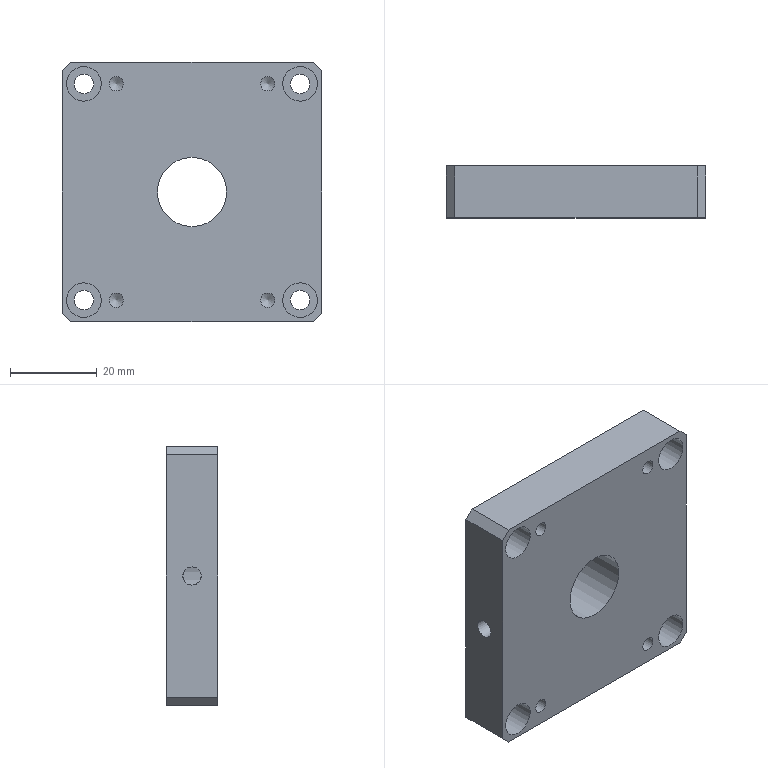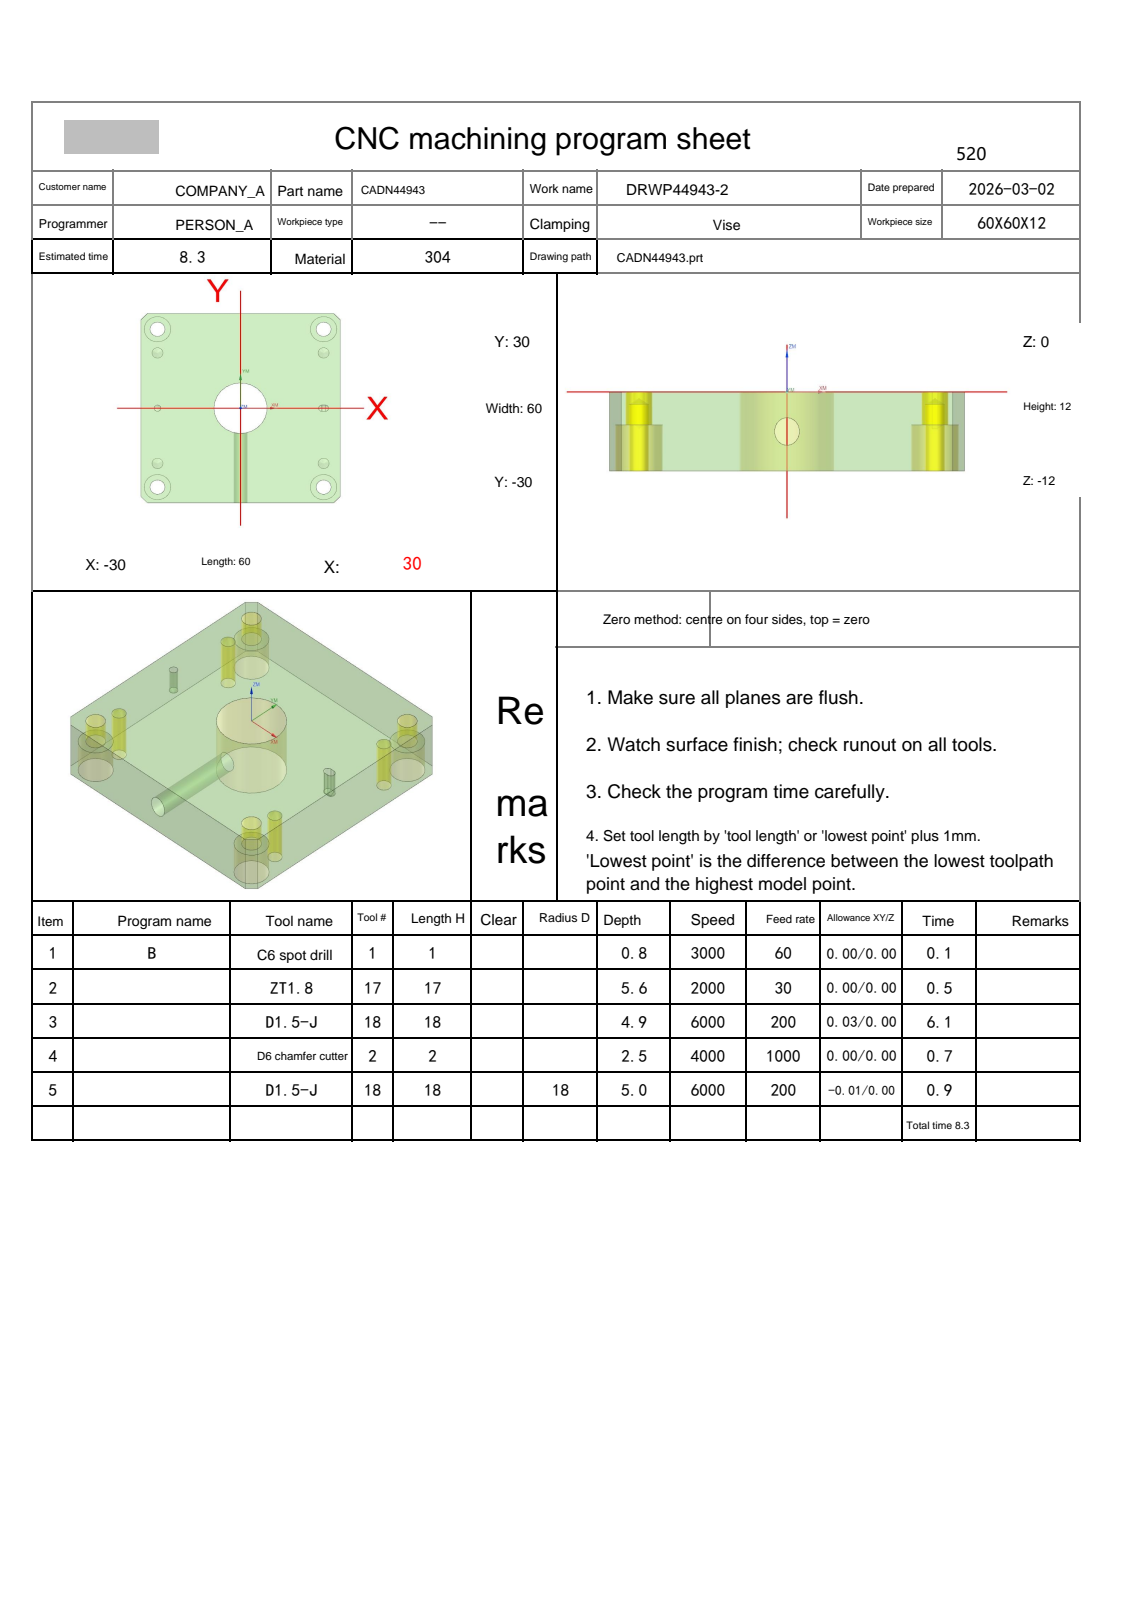NC program | NX | posted by the shop | part box 60 x 12 x 60 mm
Lines 2670 to 3254 of 3254:
N4 T02 M06
(D6 chamfer cutter  D=6. R=0. H=02 ce=0.00 di=0.00)
G00 G90 G54 X-25. Y-25. M03 S2000
G43 H02 Z50.
M08
G98 G81 X-25. Y-25. Z-2.55 R3. F100.
Y25.
X25.
Y-25.
G80
G00 Z50.
G00 G90 X-.386 Y31.227 M03 S3500
Z50.
Z.172
G01 Z-1.2 F1000.
G03 X-.1 Y31.027 I1.286 J1.532
G01 X-.054 Y30.997
X0.0 Y31.
X28.
X28.259 Y30.966
X28.5 Y30.866
X28.707 Y30.707
X30.707 Y28.707
X30.866 Y28.5
X30.966 Y28.259
X31. Y28.
Y-28.
X30.966 Y-28.259
X30.866 Y-28.5
X30.707 Y-28.707
X28.707 Y-30.707
X28.5 Y-30.866
X28.259 Y-30.966
X28. Y-31.
X-28.
X-28.259 Y-30.966
X-28.5 Y-30.866
X-28.707 Y-30.707
X-30.707 Y-28.707
X-30.866 Y-28.5
X-30.966 Y-28.259
X-31. Y-28.
Y28.
X-30.966 Y28.259
X-30.866 Y28.5
X-30.707 Y28.707
X-28.707 Y30.707
X-28.5 Y30.866
X-28.259 Y30.966
X-28. Y31.
X0.0
X.054 Y30.997
X.1 Y31.027
G03 X.386 Y31.227 I-1. J1.732
G01 Z.172
G00 Z10.
X-26.065 Y25.407
Z.294
G01 Z-1.2
G03 X-26.234 Y25.102 I1.658 J-1.118
G01 X-26.259 Y25.054
X-26.25 Y25.
G03 X-25. Y23.75 I1.25 J0.0
X-23.75 Y25. I0.0 J1.25
X-25. Y26.25 I-1.25 J0.0
X-26.223 Y25.26 I0.0 J-1.25
G01 X-26.25 Y25.
X-26.259 Y24.946
X-26.234 Y24.898
G03 X-26.065 Y24.593 I1.827 J.813
G01 Z.294
G00 Z10.
X23.935 Y25.407
Z.294
G01 Z-1.2
G03 X23.766 Y25.102 I1.658 J-1.118
G01 X23.741 Y25.054
X23.75 Y25.
G03 X25. Y23.75 I1.25 J0.0
X26.25 Y25. I0.0 J1.25
X25. Y26.25 I-1.25 J0.0
X23.777 Y25.26 I0.0 J-1.25
G01 X23.75 Y25.
X23.741 Y24.946
X23.766 Y24.898
G03 X23.935 Y24.593 I1.827 J.813
G01 Z.294
G00 Z10.
X25.116 Y-.068
Z.467
G01 Z-1.2
X25.03 Y-.008
X25. Y0.0
X24.5
X25.5
X25.
X24.97 Y-.008
X24.884 Y-.068
Z.467
G00 Z10.
X23.935 Y-24.593
Z.294
G01 Z-1.2
G03 X23.766 Y-24.898 I1.658 J-1.118
G01 X23.741 Y-24.946
X23.75 Y-25.
G03 X25. Y-26.25 I1.25 J0.0
X26.25 Y-25. I0.0 J1.25
X25. Y-23.75 I-1.25 J0.0
X23.777 Y-24.74 I0.0 J-1.25
G01 X23.75 Y-25.
X23.741 Y-25.054
X23.766 Y-25.102
G03 X23.935 Y-25.407 I1.827 J.813
G01 Z.294
G00 Z10.
X6.794 Y-.397
Z.208
G01 Z-1.2
G03 X6.978 Y-.101 I-1.597 J1.204
G01 X7.006 Y-.054
X7. Y0.0
G03 X0.0 Y7. I-7. J0.0
X-7. Y0.0 I0.0 J-7.
X0.0 Y-7. I7. J0.0
X7. Y0.0 I0.0 J7.
G01 X7.006 Y.054
X6.978 Y.101
G03 X6.794 Y.397 I-1.782 J-.908
G01 Z.208
G00 Z10.
X-26.065 Y-24.593
Z.294
G01 Z-1.2
G03 X-26.234 Y-24.898 I1.658 J-1.118
G01 X-26.259 Y-24.946
X-26.25 Y-25.
G03 X-25. Y-26.25 I1.25 J0.0
X-23.75 Y-25. I0.0 J1.25
X-25. Y-23.75 I-1.25 J0.0
X-26.223 Y-24.74 I0.0 J-1.25
G01 X-26.25 Y-25.
X-26.259 Y-25.054
X-26.234 Y-25.102
G03 X-26.065 Y-25.407 I1.827 J.813
G01 Z.294
G00 Z50.
G00 G90 X-25. Y0.0 M03 S4000
Z50.
G98 G81 X-25. Y0.0 Z-1.3 R3. F80.
G80
G00 Z50.
G91 G28 Z0.0
M05
M09
G91 G28 Z0.0
M01
N5 T18 M06
(D1.5-J  D=1.5 R=0. H=18 ce=-0.01 di=0.00)
G00 G90 G54 X25.254 Y-.227 M03 S6000
G43 H18 Z50.
M08
Z.5
G01 X25.548 Z.485 F200.
X25.664 Y-.164 Z.478
X25.727 Y-.048 Z.471
Y.048 Z.466
X25.664 Y.164 Z.459
X25.548 Y.227 Z.452
X24.452 Z.394
X24.336 Y.164 Z.387
X24.273 Y.048 Z.38
Y-.048 Z.375
X24.323 Y-.151 Z.369
X24.417 Y-.217 Z.363
X24.5 Y-.227 Z.359
X25.548 Z.304
X25.664 Y-.164 Z.297
X25.727 Y-.048 Z.29
Y.048 Z.285
X25.664 Y.164 Z.278
X25.548 Y.227 Z.271
X24.452 Z.214
X24.336 Y.164 Z.207
X24.273 Y.048 Z.2
Y-.048 Z.195
X24.323 Y-.151 Z.189
X24.417 Y-.217 Z.183
X24.5 Y-.227 Z.179
X25.548 Z.124
X25.664 Y-.164 Z.117
X25.727 Y-.048 Z.11
Y.048 Z.105
X25.664 Y.164 Z.098
X25.548 Y.227 Z.091
X24.452 Z.033
X24.336 Y.164 Z.027
X24.273 Y.048 Z.02
Y-.048 Z.015
X24.323 Y-.151 Z.009
X24.417 Y-.217 Z.003
X24.465 Y-.225 Z0.0
G41 D18
X24.5 Y-.26
X25.5 Z-.053
G03 X25.76 Y0.0 Z-.075 I0.0 J.26
X25.5 Y.26 Z-.096 I-.26 J0.0
G01 X24.5 Z-.149
G03 X24.24 Y0.0 Z-.171 I0.0 J-.26
X24.5 Y-.26 Z-.192 I.26 J0.0
G01 X25.5 Z-.245
G03 X25.76 Y0.0 Z-.267 I0.0 J.26
X25.5 Y.26 Z-.288 I-.26 J0.0
G01 X24.5 Z-.341
G03 X24.24 Y0.0 Z-.363 I0.0 J-.26
X24.5 Y-.26 Z-.385 I.26 J0.0
G01 X25.5 Z-.438
G03 X25.76 Y0.0 Z-.459 I0.0 J.26
X25.5 Y.26 Z-.481 I-.26 J0.0
G01 X24.5 Z-.534
G03 X24.24 Y0.0 Z-.555 I0.0 J-.26
X24.5 Y-.26 Z-.577 I.26 J0.0
G01 X25.5 Z-.63
G03 X25.76 Y0.0 Z-.651 I0.0 J.26
X25.5 Y.26 Z-.673 I-.26 J0.0
G01 X24.5 Z-.726
G03 X24.24 Y0.0 Z-.748 I0.0 J-.26
X24.5 Y-.26 Z-.769 I.26 J0.0
G01 X25.5 Z-.822
G03 X25.76 Y0.0 Z-.844 I0.0 J.26
X25.5 Y.26 Z-.865 I-.26 J0.0
G01 X24.5 Z-.918
G03 X24.24 Y0.0 Z-.94 I0.0 J-.26
X24.5 Y-.26 Z-.962 I.26 J0.0
G01 X25.5 Z-1.014
G03 X25.76 Y0.0 Z-1.036 I0.0 J.26
X25.5 Y.26 Z-1.058 I-.26 J0.0
G01 X24.5 Z-1.111
G03 X24.24 Y0.0 Z-1.132 I0.0 J-.26
X24.5 Y-.26 Z-1.154 I.26 J0.0
G01 X25.5 Z-1.207
G03 X25.76 Y0.0 Z-1.228 I0.0 J.26
X25.5 Y.26 Z-1.25 I-.26 J0.0
G01 X24.5 Z-1.303
G03 X24.24 Y0.0 Z-1.325 I0.0 J-.26
X24.5 Y-.26 Z-1.346 I.26 J0.0
G01 X25.5 Z-1.399
G03 X25.76 Y0.0 Z-1.421 I0.0 J.26
X25.5 Y.26 Z-1.442 I-.26 J0.0
G01 X24.5 Z-1.495
G03 X24.24 Y0.0 Z-1.517 I0.0 J-.26
X24.5 Y-.26 Z-1.538 I.26 J0.0
G01 X25.5 Z-1.591
G03 X25.76 Y0.0 Z-1.613 I0.0 J.26
X25.5 Y.26 Z-1.635 I-.26 J0.0
G01 X24.5 Z-1.688
G03 X24.24 Y0.0 Z-1.709 I0.0 J-.26
X24.5 Y-.26 Z-1.731 I.26 J0.0
G01 X25.5 Z-1.784
G03 X25.76 Y0.0 Z-1.805 I0.0 J.26
X25.5 Y.26 Z-1.827 I-.26 J0.0
G01 X24.5 Z-1.88
G03 X24.24 Y0.0 Z-1.901 I0.0 J-.26
X24.5 Y-.26 Z-1.923 I.26 J0.0
G01 X25.5 Z-1.976
G03 X25.76 Y0.0 Z-1.998 I0.0 J.26
X25.5 Y.26 Z-2.019 I-.26 J0.0
G01 X24.5 Z-2.072
G03 X24.24 Y0.0 Z-2.094 I0.0 J-.26
X24.5 Y-.26 Z-2.115 I.26 J0.0
G01 X25.5 Z-2.168
G03 X25.76 Y0.0 Z-2.19 I0.0 J.26
X25.5 Y.26 Z-2.212 I-.26 J0.0
G01 X24.5 Z-2.264
G03 X24.24 Y0.0 Z-2.286 I0.0 J-.26
X24.5 Y-.26 Z-2.308 I.26 J0.0
G01 X25.5 Z-2.361
G03 X25.76 Y0.0 Z-2.382 I0.0 J.26
X25.5 Y.26 Z-2.404 I-.26 J0.0
G01 X24.5 Z-2.457
G03 X24.24 Y0.0 Z-2.478 I0.0 J-.26
X24.5 Y-.26 Z-2.5 I.26 J0.0
G01 X25.5 Z-2.553
G03 X25.76 Y0.0 Z-2.575 I0.0 J.26
X25.5 Y.26 Z-2.596 I-.26 J0.0
G01 X24.5 Z-2.649
G03 X24.24 Y0.0 Z-2.671 I0.0 J-.26
X24.5 Y-.26 Z-2.692 I.26 J0.0
G01 X25.5 Z-2.745
G03 X25.76 Y0.0 Z-2.767 I0.0 J.26
X25.5 Y.26 Z-2.788 I-.26 J0.0
G01 X24.5 Z-2.841
G03 X24.24 Y0.0 Z-2.863 I0.0 J-.26
X24.5 Y-.26 Z-2.885 I.26 J0.0
G01 X25.5 Z-2.938
G03 X25.76 Y0.0 Z-2.959 I0.0 J.26
X25.5 Y.26 Z-2.981 I-.26 J0.0
G01 X24.5 Z-3.034
G03 X24.24 Y0.0 Z-3.055 I0.0 J-.26
X24.5 Y-.26 Z-3.077 I.26 J0.0
G01 X25.5 Z-3.13
G03 X25.76 Y0.0 Z-3.151 I0.0 J.26
X25.5 Y.26 Z-3.173 I-.26 J0.0
G01 X24.5 Z-3.226
G03 X24.24 Y0.0 Z-3.248 I0.0 J-.26
X24.5 Y-.26 Z-3.269 I.26 J0.0
G01 X25.5 Z-3.322
G03 X25.76 Y0.0 Z-3.344 I0.0 J.26
X25.5 Y.26 Z-3.365 I-.26 J0.0
G01 X24.5 Z-3.418
G03 X24.24 Y0.0 Z-3.44 I0.0 J-.26
X24.5 Y-.26 Z-3.462 I.26 J0.0
G01 X25.5 Z-3.514
G03 X25.76 Y0.0 Z-3.536 I0.0 J.26
X25.5 Y.26 Z-3.558 I-.26 J0.0
G01 X24.5 Z-3.611
G03 X24.24 Y0.0 Z-3.632 I0.0 J-.26
X24.5 Y-.26 Z-3.654 I.26 J0.0
G01 X25.5 Z-3.707
G03 X25.76 Y0.0 Z-3.728 I0.0 J.26
X25.5 Y.26 Z-3.75 I-.26 J0.0
G01 X24.5 Z-3.803
G03 X24.24 Y0.0 Z-3.825 I0.0 J-.26
X24.5 Y-.26 Z-3.846 I.26 J0.0
G01 X25.5 Z-3.899
G03 X25.76 Y0.0 Z-3.921 I0.0 J.26
X25.5 Y.26 Z-3.942 I-.26 J0.0
G01 X24.5 Z-3.995
G03 X24.24 Y0.0 Z-4.017 I0.0 J-.26
X24.5 Y-.26 Z-4.038 I.26 J0.0
G01 X25.5 Z-4.091
G03 X25.76 Y0.0 Z-4.113 I0.0 J.26
X25.5 Y.26 Z-4.135 I-.26 J0.0
G01 X24.5 Z-4.188
G03 X24.24 Y0.0 Z-4.209 I0.0 J-.26
X24.5 Y-.26 Z-4.231 I.26 J0.0
G01 X25.5 Z-4.284
G03 X25.76 Y0.0 Z-4.305 I0.0 J.26
X25.5 Y.26 Z-4.327 I-.26 J0.0
G01 X24.5 Z-4.38
G03 X24.24 Y0.0 Z-4.401 I0.0 J-.26
X24.5 Y-.26 Z-4.423 I.26 J0.0
G01 X25.5 Z-4.476
G03 X25.76 Y0.0 Z-4.498 I0.0 J.26
X25.5 Y.26 Z-4.519 I-.26 J0.0
G01 X24.5 Z-4.572
G03 X24.24 Y0.0 Z-4.594 I0.0 J-.26
X24.5 Y-.26 Z-4.615 I.26 J0.0
G01 X25.5 Z-4.668
G03 X25.76 Y0.0 Z-4.69 I0.0 J.26
X25.5 Y.26 Z-4.712 I-.26 J0.0
G01 X24.5 Z-4.764
G03 X24.24 Y0.0 Z-4.786 I0.0 J-.26
X24.5 Y-.26 Z-4.808 I.26 J0.0
G01 X25.5 Z-4.861
G03 X25.76 Y0.0 Z-4.882 I0.0 J.26
X25.5 Y.26 Z-4.904 I-.26 J0.0
G01 X24.5 Z-4.957
G03 X24.24 Y0.0 Z-4.978 I0.0 J-.26
X24.5 Y-.26 Z-5. I.26 J0.0
G01 X25.5
G03 X25.76 Y0.0 I0.0 J.26
X25.5 Y.26 I-.26 J0.0
G01 X24.5
G03 X24.24 Y0.0 I0.0 J-.26
X24.5 Y-.26 I.26 J0.0
G01 X24.9
X24.928 Y-.258
X24.948 Y-.238
X24.95 Y-.21
G40 Y-.16
Z-4.
G00 Z50.
X-24.848 Y-.171
Z.5
G01 X-24.836 Y-.164 Z.499
X-24.773 Y-.048 Z.492
Y.048 Z.487
X-24.836 Y.164 Z.48
X-24.952 Y.227 Z.473
X-25.048 Z.468
X-25.151 Y.177 Z.462
X-25.217 Y.083 Z.456
X-25.227 Y0.0 Z.452
Y-.048 Z.449
X-25.164 Y-.164 Z.443
X-25.048 Y-.227 Z.436
X-24.952 Z.431
X-24.836 Y-.164 Z.424
X-24.773 Y-.048 Z.417
Y.048 Z.412
X-24.836 Y.164 Z.405
X-24.952 Y.227 Z.398
X-25.048 Z.393
X-25.151 Y.177 Z.387
X-25.217 Y.083 Z.381
X-25.227 Y0.0 Z.376
Y-.048 Z.374
X-25.164 Y-.164 Z.367
X-25.048 Y-.227 Z.36
X-24.952 Z.355
X-24.836 Y-.164 Z.348
X-24.773 Y-.048 Z.341
Y.048 Z.336
X-24.836 Y.164 Z.329
X-24.952 Y.227 Z.322
X-25.048 Z.317
X-25.151 Y.177 Z.311
X-25.217 Y.083 Z.305
X-25.227 Y0.0 Z.301
Y-.048 Z.298
X-25.164 Y-.164 Z.291
X-25.048 Y-.227 Z.284
X-24.952 Z.279
X-24.836 Y-.164 Z.272
X-24.773 Y-.048 Z.265
Y.048 Z.26
X-24.836 Y.164 Z.253
X-24.952 Y.227 Z.246
X-25.048 Z.241
X-25.151 Y.177 Z.235
X-25.217 Y.083 Z.229
X-25.227 Y0.0 Z.225
Y-.048 Z.223
X-25.164 Y-.164 Z.216
X-25.048 Y-.227 Z.209
X-24.952 Z.204
X-24.836 Y-.164 Z.197
X-24.773 Y-.048 Z.19
Y.048 Z.185
X-24.836 Y.164 Z.178
X-24.952 Y.227 Z.171
X-25.048 Z.166
X-25.151 Y.177 Z.16
X-25.217 Y.083 Z.154
X-25.227 Y0.0 Z.149
Y-.048 Z.147
X-25.164 Y-.164 Z.14
X-25.048 Y-.227 Z.133
X-24.952 Z.128
X-24.836 Y-.164 Z.121
X-24.773 Y-.048 Z.114
Y.048 Z.109
X-24.836 Y.164 Z.102
X-24.952 Y.227 Z.095
X-25.048 Z.09
X-25.151 Y.177 Z.084
X-25.217 Y.083 Z.078
X-25.227 Y0.0 Z.074
Y-.048 Z.071
X-25.164 Y-.164 Z.064
X-25.048 Y-.227 Z.057
X-24.952 Z.052
X-24.836 Y-.164 Z.045
X-24.773 Y-.048 Z.038
Y.048 Z.033
X-24.836 Y.164 Z.027
X-24.952 Y.227 Z.02
X-25.048 Z.015
X-25.151 Y.177 Z.009
X-25.217 Y.083 Z.003
X-25.225 Y.035 Z0.0
G41 D18
X-25.26 Y0.0
G03 X-25. Y-.26 Z-.048 I.26 J0.0
X-24.74 Y0.0 Z-.096 I0.0 J.26
X-25. Y.26 Z-.144 I-.26 J0.0
X-25.26 Y0.0 Z-.192 I0.0 J-.26
X-25. Y-.26 Z-.24 I.26 J0.0
X-24.74 Y0.0 Z-.288 I0.0 J.26
X-25. Y.26 Z-.337 I-.26 J0.0
X-25.26 Y0.0 Z-.385 I0.0 J-.26
X-25. Y-.26 Z-.433 I.26 J0.0
X-24.74 Y0.0 Z-.481 I0.0 J.26
X-25. Y.26 Z-.529 I-.26 J0.0
X-25.26 Y0.0 Z-.577 I0.0 J-.26
X-25. Y-.26 Z-.625 I.26 J0.0
X-24.74 Y0.0 Z-.673 I0.0 J.26
X-25. Y.26 Z-.721 I-.26 J0.0
X-25.26 Y0.0 Z-.769 I0.0 J-.26
X-25. Y-.26 Z-.817 I.26 J0.0
X-24.74 Y0.0 Z-.865 I0.0 J.26
X-25. Y.26 Z-.913 I-.26 J0.0
X-25.26 Y0.0 Z-.962 I0.0 J-.26
X-25. Y-.26 Z-1.01 I.26 J0.0
X-24.74 Y0.0 Z-1.058 I0.0 J.26
X-25. Y.26 Z-1.106 I-.26 J0.0
X-25.26 Y0.0 Z-1.154 I0.0 J-.26
X-25. Y-.26 Z-1.202 I.26 J0.0
X-24.74 Y0.0 Z-1.25 I0.0 J.26
X-25. Y.26 Z-1.298 I-.26 J0.0
X-25.26 Y0.0 Z-1.346 I0.0 J-.26
X-25. Y-.26 Z-1.394 I.26 J0.0
X-24.74 Y0.0 Z-1.442 I0.0 J.26
X-25. Y.26 Z-1.49 I-.26 J0.0
X-25.26 Y0.0 Z-1.538 I0.0 J-.26
X-25. Y-.26 Z-1.587 I.26 J0.0
X-24.74 Y0.0 Z-1.635 I0.0 J.26
X-25. Y.26 Z-1.683 I-.26 J0.0
X-25.26 Y0.0 Z-1.731 I0.0 J-.26
X-25. Y-.26 Z-1.779 I.26 J0.0
X-24.74 Y0.0 Z-1.827 I0.0 J.26
X-25. Y.26 Z-1.875 I-.26 J0.0
X-25.26 Y0.0 Z-1.923 I0.0 J-.26
X-25. Y-.26 Z-1.971 I.26 J0.0
X-24.74 Y0.0 Z-2.019 I0.0 J.26
X-25. Y.26 Z-2.067 I-.26 J0.0
X-25.26 Y0.0 Z-2.115 I0.0 J-.26
X-25. Y-.26 Z-2.163 I.26 J0.0
X-24.74 Y0.0 Z-2.212 I0.0 J.26
X-25. Y.26 Z-2.26 I-.26 J0.0
X-25.26 Y0.0 Z-2.308 I0.0 J-.26
X-25. Y-.26 Z-2.356 I.26 J0.0
X-24.74 Y0.0 Z-2.404 I0.0 J.26
X-25. Y.26 Z-2.452 I-.26 J0.0
X-25.26 Y0.0 Z-2.5 I0.0 J-.26
X-25. Y-.26 Z-2.548 I.26 J0.0
X-24.74 Y0.0 Z-2.596 I0.0 J.26
X-25. Y.26 Z-2.644 I-.26 J0.0
X-25.26 Y0.0 Z-2.692 I0.0 J-.26
X-25. Y-.26 Z-2.74 I.26 J0.0
X-24.74 Y0.0 Z-2.788 I0.0 J.26
X-25. Y.26 Z-2.837 I-.26 J0.0
X-25.26 Y0.0 Z-2.885 I0.0 J-.26
X-25. Y-.26 Z-2.933 I.26 J0.0
X-24.74 Y0.0 Z-2.981 I0.0 J.26
X-25. Y.26 Z-3.029 I-.26 J0.0
X-25.26 Y0.0 Z-3.077 I0.0 J-.26
X-25. Y-.26 Z-3.125 I.26 J0.0
X-24.74 Y0.0 Z-3.173 I0.0 J.26
X-25. Y.26 Z-3.221 I-.26 J0.0
X-25.26 Y0.0 Z-3.269 I0.0 J-.26
X-25. Y-.26 Z-3.317 I.26 J0.0
X-24.74 Y0.0 Z-3.365 I0.0 J.26
X-25. Y.26 Z-3.413 I-.26 J0.0
X-25.26 Y0.0 Z-3.462 I0.0 J-.26
X-25. Y-.26 Z-3.51 I.26 J0.0
X-24.74 Y0.0 Z-3.558 I0.0 J.26
X-25. Y.26 Z-3.606 I-.26 J0.0
X-25.26 Y0.0 Z-3.654 I0.0 J-.26
X-25. Y-.26 Z-3.702 I.26 J0.0
X-24.74 Y0.0 Z-3.75 I0.0 J.26
X-25. Y.26 Z-3.798 I-.26 J0.0
X-25.26 Y0.0 Z-3.846 I0.0 J-.26
X-25. Y-.26 Z-3.894 I.26 J0.0
X-24.74 Y0.0 Z-3.942 I0.0 J.26
X-25. Y.26 Z-3.99 I-.26 J0.0
X-25.26 Y0.0 Z-4.038 I0.0 J-.26
X-25. Y-.26 Z-4.087 I.26 J0.0
X-24.74 Y0.0 Z-4.135 I0.0 J.26
X-25. Y.26 Z-4.183 I-.26 J0.0
X-25.26 Y0.0 Z-4.231 I0.0 J-.26
X-25. Y-.26 Z-4.279 I.26 J0.0
X-24.74 Y0.0 Z-4.327 I0.0 J.26
X-25. Y.26 Z-4.375 I-.26 J0.0
X-25.26 Y0.0 Z-4.423 I0.0 J-.26
X-25. Y-.26 Z-4.471 I.26 J0.0
X-24.74 Y0.0 Z-4.519 I0.0 J.26
X-25. Y.26 Z-4.567 I-.26 J0.0
X-25.26 Y0.0 Z-4.615 I0.0 J-.26
X-25. Y-.26 Z-4.663 I.26 J0.0
X-24.74 Y0.0 Z-4.712 I0.0 J.26
X-25. Y.26 Z-4.76 I-.26 J0.0
X-25.26 Y0.0 Z-4.808 I0.0 J-.26
X-25. Y-.26 Z-4.856 I.26 J0.0
X-24.74 Y0.0 Z-4.904 I0.0 J.26
X-25. Y.26 Z-4.952 I-.26 J0.0
X-25.26 Y0.0 Z-5. I0.0 J-.26
X-25. Y-.26 I.26 J0.0
X-24.74 Y0.0 I0.0 J.26
X-25. Y.26 I-.26 J0.0
X-25.26 Y0.0 I0.0 J-.26
X-25.008 Y-.26 I.26 J0.0
G01 X-24.981 Y-.258
X-24.96 Y-.239
X-24.957 Y-.212
G40 X-24.955 Y-.162
Z-4.
G00 Z50.
M05
M09
G91 G28 Z0.0
G91 G28 Y0.0
M30
%